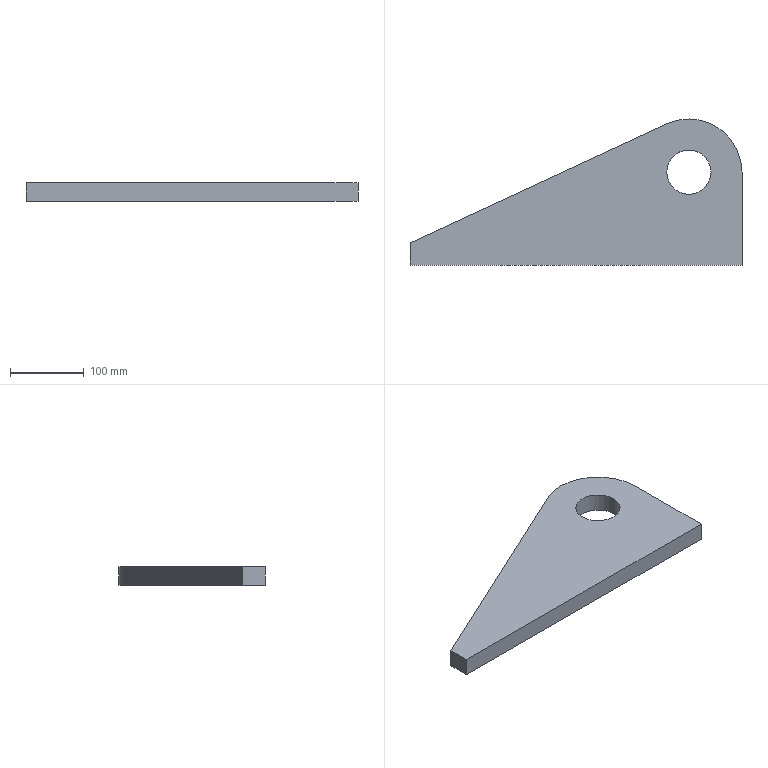Part | SolidWorks | features Extrusion 1 | 1 solid | 9 faces | box 450 x 198 x 25 mm | volume 1368117 mm3 | plane 6 | cylinder 3 | commonest cylinder face diameters 60 x2 144 x1
STEP:
#1=CARTESIAN_POINT('',(348.,126.,25.));
#2=VERTEX_POINT('',#1);
#3=CARTESIAN_POINT('',(408.,126.,25.));
#4=VERTEX_POINT('',#3);
#5=CARTESIAN_POINT('',(378.,126.,25.));
#6=DIRECTION('',(0.,0.,1.));
#7=DIRECTION('',(1.,0.,0.));
#8=AXIS2_PLACEMENT_3D('',#5,#6,#7);
#9=CIRCLE('',#8,30.);
#10=EDGE_CURVE('',#2,#4,#9,.T.);
#11=ORIENTED_EDGE('',*,*,#10,.T.);
#12=CARTESIAN_POINT('',(408.,126.,0.));
#13=VERTEX_POINT('',#12);
#14=CARTESIAN_POINT('',(408.,126.,25.));
#15=DIRECTION('',(0.,0.,-1.));
#16=VECTOR('',#15,1000.);
#17=LINE('',#14,#16);
#18=EDGE_CURVE('',#4,#13,#17,.T.);
#19=ORIENTED_EDGE('',*,*,#18,.T.);
#20=CARTESIAN_POINT('',(348.,126.,0.));
#21=VERTEX_POINT('',#20);
#22=CARTESIAN_POINT('',(378.,126.,0.));
#23=DIRECTION('',(0.,0.,1.));
#24=DIRECTION('',(1.,0.,0.));
#25=AXIS2_PLACEMENT_3D('',#22,#23,#24);
#26=CIRCLE('',#25,30.);
#27=EDGE_CURVE('',#21,#13,#26,.T.);
#28=ORIENTED_EDGE('',*,*,#27,.F.);
#29=CARTESIAN_POINT('',(348.,126.,25.));
#30=DIRECTION('',(0.,0.,-1.));
#31=VECTOR('',#30,1000.);
#32=LINE('',#29,#31);
#33=EDGE_CURVE('',#2,#21,#32,.T.);
#34=ORIENTED_EDGE('',*,*,#33,.F.);
#35=EDGE_LOOP('',(#11,#19,#28,#34));
#36=FACE_OUTER_BOUND('',#35,.T.);
#37=CARTESIAN_POINT('',(378.,126.,25.));
#38=DIRECTION('',(0.,0.,-1.));
#39=DIRECTION('',(-1.,0.,0.));
#40=AXIS2_PLACEMENT_3D('',#37,#38,#39);
#41=CYLINDRICAL_SURFACE('',#40,30.);
#42=ADVANCED_FACE('',(#36),#41,.F.);
#43=CARTESIAN_POINT('',(0.,0.,25.));
#44=VERTEX_POINT('',#43);
#45=CARTESIAN_POINT('',(450.,0.,25.));
#46=VERTEX_POINT('',#45);
#47=CARTESIAN_POINT('',(450.,0.,25.));
#48=DIRECTION('',(1.,0.,0.));
#49=VECTOR('',#48,1000.);
#50=LINE('',#47,#49);
#51=EDGE_CURVE('',#44,#46,#50,.T.);
#52=ORIENTED_EDGE('',*,*,#51,.T.);
#53=CARTESIAN_POINT('',(450.,126.,25.));
#54=VERTEX_POINT('',#53);
#55=CARTESIAN_POINT('',(450.,126.,25.));
#56=DIRECTION('',(0.,1.,0.));
#57=VECTOR('',#56,1000.);
#58=LINE('',#55,#57);
#59=EDGE_CURVE('',#46,#54,#58,.T.);
#60=ORIENTED_EDGE('',*,*,#59,.T.);
#61=CARTESIAN_POINT('',(347.698,191.313,25.));
#62=VERTEX_POINT('',#61);
#63=CARTESIAN_POINT('',(378.,126.,25.));
#64=DIRECTION('',(0.,0.,1.));
#65=DIRECTION('',(-1.,0.,0.));
#66=AXIS2_PLACEMENT_3D('',#63,#64,#65);
#67=CIRCLE('',#66,72.);
#68=EDGE_CURVE('',#54,#62,#67,.T.);
#69=ORIENTED_EDGE('',*,*,#68,.T.);
#70=CARTESIAN_POINT('',(0.,30.,25.));
#71=VERTEX_POINT('',#70);
#72=CARTESIAN_POINT('',(0.,30.,25.));
#73=DIRECTION('',(-0.9071,-0.4209,0.));
#74=VECTOR('',#73,1000.);
#75=LINE('',#72,#74);
#76=EDGE_CURVE('',#62,#71,#75,.T.);
#77=ORIENTED_EDGE('',*,*,#76,.T.);
#78=CARTESIAN_POINT('',(0.,0.,25.));
#79=DIRECTION('',(0.,-1.,0.));
#80=VECTOR('',#79,1000.);
#81=LINE('',#78,#80);
#82=EDGE_CURVE('',#71,#44,#81,.T.);
#83=ORIENTED_EDGE('',*,*,#82,.T.);
#84=EDGE_LOOP('',(#52,#60,#69,#77,#83));
#85=FACE_OUTER_BOUND('',#84,.T.);
#86=ORIENTED_EDGE('',*,*,#10,.F.);
#87=CARTESIAN_POINT('',(378.,126.,25.));
#88=DIRECTION('',(0.,0.,1.));
#89=DIRECTION('',(1.,0.,0.));
#90=AXIS2_PLACEMENT_3D('',#87,#88,#89);
#91=CIRCLE('',#90,30.);
#92=EDGE_CURVE('',#4,#2,#91,.T.);
#93=ORIENTED_EDGE('',*,*,#92,.F.);
#94=EDGE_LOOP('',(#86,#93));
#95=FACE_BOUND('',#94,.T.);
#96=CARTESIAN_POINT('',(378.,126.,25.));
#97=DIRECTION('',(0.,0.,-1.));
#98=DIRECTION('',(-1.,0.,0.));
#99=AXIS2_PLACEMENT_3D('',#96,#97,#98);
#100=PLANE('',#99);
#101=ADVANCED_FACE('',(#85,#95),#100,.F.);
#102=CARTESIAN_POINT('',(0.,0.,0.));
#103=VERTEX_POINT('',#102);
#104=CARTESIAN_POINT('',(450.,0.,0.));
#105=VERTEX_POINT('',#104);
#106=CARTESIAN_POINT('',(450.,0.,0.));
#107=DIRECTION('',(1.,0.,0.));
#108=VECTOR('',#107,1000.);
#109=LINE('',#106,#108);
#110=EDGE_CURVE('',#103,#105,#109,.T.);
#111=ORIENTED_EDGE('',*,*,#110,.F.);
#112=CARTESIAN_POINT('',(0.,30.,0.));
#113=VERTEX_POINT('',#112);
#114=CARTESIAN_POINT('',(0.,0.,0.));
#115=DIRECTION('',(0.,-1.,0.));
#116=VECTOR('',#115,1000.);
#117=LINE('',#114,#116);
#118=EDGE_CURVE('',#113,#103,#117,.T.);
#119=ORIENTED_EDGE('',*,*,#118,.F.);
#120=CARTESIAN_POINT('',(347.698,191.313,0.));
#121=VERTEX_POINT('',#120);
#122=CARTESIAN_POINT('',(0.,30.,0.));
#123=DIRECTION('',(-0.9071,-0.4209,0.));
#124=VECTOR('',#123,1000.);
#125=LINE('',#122,#124);
#126=EDGE_CURVE('',#121,#113,#125,.T.);
#127=ORIENTED_EDGE('',*,*,#126,.F.);
#128=CARTESIAN_POINT('',(450.,126.,0.));
#129=VERTEX_POINT('',#128);
#130=CARTESIAN_POINT('',(378.,126.,0.));
#131=DIRECTION('',(0.,0.,1.));
#132=DIRECTION('',(-1.,0.,0.));
#133=AXIS2_PLACEMENT_3D('',#130,#131,#132);
#134=CIRCLE('',#133,72.);
#135=EDGE_CURVE('',#129,#121,#134,.T.);
#136=ORIENTED_EDGE('',*,*,#135,.F.);
#137=CARTESIAN_POINT('',(450.,126.,0.));
#138=DIRECTION('',(0.,1.,0.));
#139=VECTOR('',#138,1000.);
#140=LINE('',#137,#139);
#141=EDGE_CURVE('',#105,#129,#140,.T.);
#142=ORIENTED_EDGE('',*,*,#141,.F.);
#143=EDGE_LOOP('',(#111,#119,#127,#136,#142));
#144=FACE_OUTER_BOUND('',#143,.T.);
#145=ORIENTED_EDGE('',*,*,#27,.T.);
#146=CARTESIAN_POINT('',(378.,126.,0.));
#147=DIRECTION('',(0.,0.,1.));
#148=DIRECTION('',(1.,0.,0.));
#149=AXIS2_PLACEMENT_3D('',#146,#147,#148);
#150=CIRCLE('',#149,30.);
#151=EDGE_CURVE('',#13,#21,#150,.T.);
#152=ORIENTED_EDGE('',*,*,#151,.T.);
#153=EDGE_LOOP('',(#145,#152));
#154=FACE_BOUND('',#153,.T.);
#155=CARTESIAN_POINT('',(378.,126.,0.));
#156=DIRECTION('',(0.,0.,-1.));
#157=DIRECTION('',(-1.,0.,0.));
#158=AXIS2_PLACEMENT_3D('',#155,#156,#157);
#159=PLANE('',#158);
#160=ADVANCED_FACE('',(#144,#154),#159,.T.);
#161=ORIENTED_EDGE('',*,*,#110,.T.);
#162=CARTESIAN_POINT('',(450.,0.,25.));
#163=DIRECTION('',(0.,0.,-1.));
#164=VECTOR('',#163,1000.);
#165=LINE('',#162,#164);
#166=EDGE_CURVE('',#46,#105,#165,.T.);
#167=ORIENTED_EDGE('',*,*,#166,.F.);
#168=ORIENTED_EDGE('',*,*,#51,.F.);
#169=CARTESIAN_POINT('',(0.,0.,25.));
#170=DIRECTION('',(0.,0.,-1.));
#171=VECTOR('',#170,1000.);
#172=LINE('',#169,#171);
#173=EDGE_CURVE('',#44,#103,#172,.T.);
#174=ORIENTED_EDGE('',*,*,#173,.T.);
#175=EDGE_LOOP('',(#161,#167,#168,#174));
#176=FACE_OUTER_BOUND('',#175,.T.);
#177=CARTESIAN_POINT('',(450.,0.,25.));
#178=DIRECTION('',(0.,1.,0.));
#179=DIRECTION('',(-1.,0.,0.));
#180=AXIS2_PLACEMENT_3D('',#177,#178,#179);
#181=PLANE('',#180);
#182=ADVANCED_FACE('',(#176),#181,.F.);
#183=ORIENTED_EDGE('',*,*,#141,.T.);
#184=CARTESIAN_POINT('',(450.,126.,25.));
#185=DIRECTION('',(0.,0.,-1.));
#186=VECTOR('',#185,1000.);
#187=LINE('',#184,#186);
#188=EDGE_CURVE('',#54,#129,#187,.T.);
#189=ORIENTED_EDGE('',*,*,#188,.F.);
#190=ORIENTED_EDGE('',*,*,#59,.F.);
#191=ORIENTED_EDGE('',*,*,#166,.T.);
#192=EDGE_LOOP('',(#183,#189,#190,#191));
#193=FACE_OUTER_BOUND('',#192,.T.);
#194=CARTESIAN_POINT('',(450.,126.,25.));
#195=DIRECTION('',(-1.,0.,0.));
#196=DIRECTION('',(0.,0.,1.));
#197=AXIS2_PLACEMENT_3D('',#194,#195,#196);
#198=PLANE('',#197);
#199=ADVANCED_FACE('',(#193),#198,.F.);
#200=ORIENTED_EDGE('',*,*,#135,.T.);
#201=CARTESIAN_POINT('',(347.698,191.313,25.));
#202=DIRECTION('',(0.,0.,-1.));
#203=VECTOR('',#202,1000.);
#204=LINE('',#201,#203);
#205=EDGE_CURVE('',#62,#121,#204,.T.);
#206=ORIENTED_EDGE('',*,*,#205,.F.);
#207=ORIENTED_EDGE('',*,*,#68,.F.);
#208=ORIENTED_EDGE('',*,*,#188,.T.);
#209=EDGE_LOOP('',(#200,#206,#207,#208));
#210=FACE_OUTER_BOUND('',#209,.T.);
#211=CARTESIAN_POINT('',(378.,126.,25.));
#212=DIRECTION('',(0.,0.,-1.));
#213=DIRECTION('',(-1.,0.,0.));
#214=AXIS2_PLACEMENT_3D('',#211,#212,#213);
#215=CYLINDRICAL_SURFACE('',#214,72.);
#216=ADVANCED_FACE('',(#210),#215,.T.);
#217=ORIENTED_EDGE('',*,*,#126,.T.);
#218=CARTESIAN_POINT('',(0.,30.,25.));
#219=DIRECTION('',(0.,0.,-1.));
#220=VECTOR('',#219,1000.);
#221=LINE('',#218,#220);
#222=EDGE_CURVE('',#71,#113,#221,.T.);
#223=ORIENTED_EDGE('',*,*,#222,.F.);
#224=ORIENTED_EDGE('',*,*,#76,.F.);
#225=ORIENTED_EDGE('',*,*,#205,.T.);
#226=EDGE_LOOP('',(#217,#223,#224,#225));
#227=FACE_OUTER_BOUND('',#226,.T.);
#228=CARTESIAN_POINT('',(0.,30.,25.));
#229=DIRECTION('',(0.4209,-0.9071,0.));
#230=DIRECTION('',(0.9071,0.4209,0.));
#231=AXIS2_PLACEMENT_3D('',#228,#229,#230);
#232=PLANE('',#231);
#233=ADVANCED_FACE('',(#227),#232,.F.);
#234=ORIENTED_EDGE('',*,*,#118,.T.);
#235=ORIENTED_EDGE('',*,*,#173,.F.);
#236=ORIENTED_EDGE('',*,*,#82,.F.);
#237=ORIENTED_EDGE('',*,*,#222,.T.);
#238=EDGE_LOOP('',(#234,#235,#236,#237));
#239=FACE_OUTER_BOUND('',#238,.T.);
#240=CARTESIAN_POINT('',(0.,0.,25.));
#241=DIRECTION('',(1.,0.,0.));
#242=DIRECTION('',(0.,0.,-1.));
#243=AXIS2_PLACEMENT_3D('',#240,#241,#242);
#244=PLANE('',#243);
#245=ADVANCED_FACE('',(#239),#244,.F.);
#246=ORIENTED_EDGE('',*,*,#18,.F.);
#247=ORIENTED_EDGE('',*,*,#92,.T.);
#248=ORIENTED_EDGE('',*,*,#33,.T.);
#249=ORIENTED_EDGE('',*,*,#151,.F.);
#250=EDGE_LOOP('',(#246,#247,#248,#249));
#251=FACE_OUTER_BOUND('',#250,.T.);
#252=CARTESIAN_POINT('',(378.,126.,25.));
#253=DIRECTION('',(0.,0.,-1.));
#254=DIRECTION('',(-1.,0.,0.));
#255=AXIS2_PLACEMENT_3D('',#252,#253,#254);
#256=CYLINDRICAL_SURFACE('',#255,30.);
#257=ADVANCED_FACE('',(#251),#256,.F.);
#258=CLOSED_SHELL('',(#42,#101,#160,#182,#199,#216,#233,#245,#257));
#259=MANIFOLD_SOLID_BREP('',#258);
#260=CARTESIAN_POINT('',(0.,0.,0.));
#261=DIRECTION('',(0.,0.,1.));
#262=DIRECTION('',(1.,0.,0.));
#263=AXIS2_PLACEMENT_3D('',#260,#261,#262);
#264=(LENGTH_UNIT()NAMED_UNIT(*)SI_UNIT(.MILLI.,.METRE.));
#265=UNCERTAINTY_MEASURE_WITH_UNIT(LENGTH_MEASURE(0.00001),#264,'','');
#266=(NAMED_UNIT(*)PLANE_ANGLE_UNIT()SI_UNIT($,.RADIAN.));
#267=(NAMED_UNIT(*)SI_UNIT($,.STERADIAN.)SOLID_ANGLE_UNIT());
#268=(GEOMETRIC_REPRESENTATION_CONTEXT(3)GLOBAL_UNCERTAINTY_ASSIGNED_CONTEXT((#265))GLOBAL_UNIT_ASSIGNED_CONTEXT((#264,#266,#267))REPRESENTATION_CONTEXT('',''));
#269=ADVANCED_BREP_SHAPE_REPRESENTATION('',(#259,#263),#268);